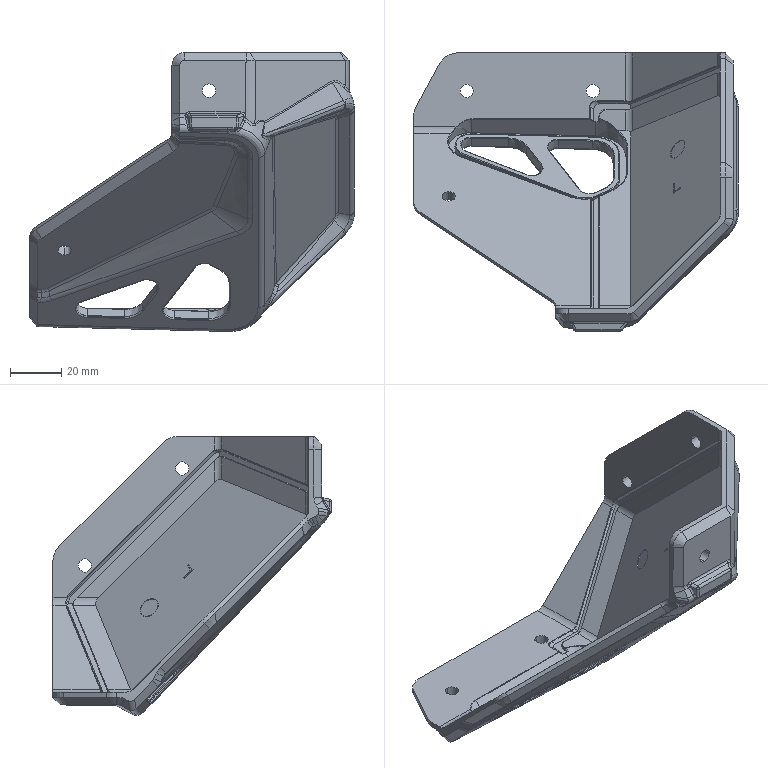Part | SolidWorks | features BaseBody 1 | 1 solid | 442 faces | box 126.894 x 108.879 x 109.039 mm | volume 93594 mm3 | spline 146 | cylinder 125 | plane 99 | cone 32 | torus 31 | sphere 9 | commonest cylinder face diameters 0.6 x31 5.2 x19 8 x19 6 x13 1 x12 10 x10